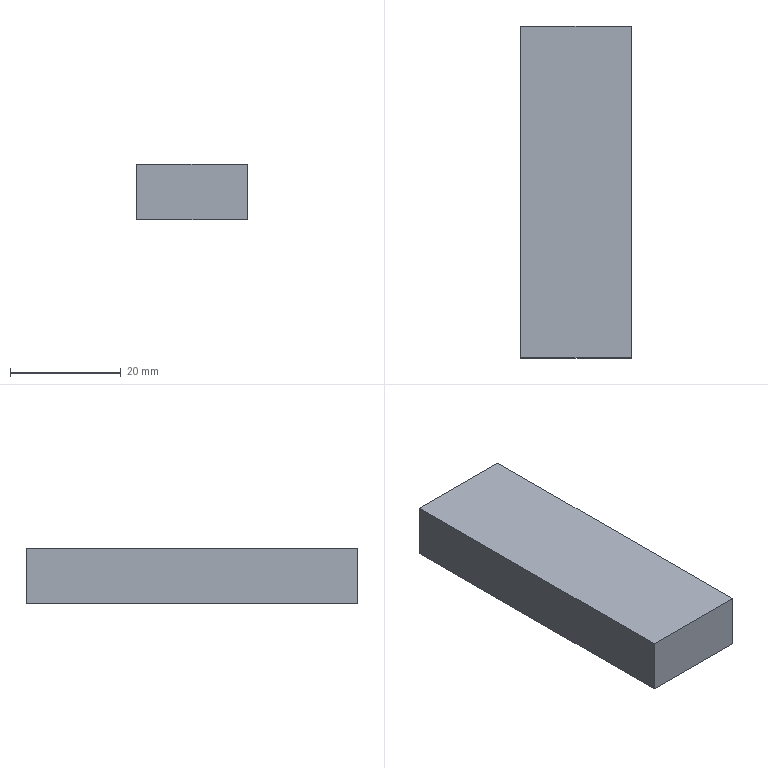Part | SolidWorks | features ICE 2, Extrusion 1 | 1 solid | 6 faces | box 20 x 60 x 10 mm | volume 12000 mm3 | plane 6
STEP:
#1=CARTESIAN_POINT('',(0.,0.,0.));
#2=VERTEX_POINT('',#1);
#3=CARTESIAN_POINT('',(20.,0.,0.));
#4=VERTEX_POINT('',#3);
#5=CARTESIAN_POINT('',(150.,0.,0.));
#6=DIRECTION('',(1.,0.,0.));
#7=VECTOR('',#6,1000.);
#8=LINE('',#5,#7);
#9=EDGE_CURVE('',#2,#4,#8,.T.);
#10=ORIENTED_EDGE('',*,*,#9,.T.);
#11=CARTESIAN_POINT('',(20.,0.,10.));
#12=VERTEX_POINT('',#11);
#13=CARTESIAN_POINT('',(20.,0.,0.));
#14=DIRECTION('',(0.,0.,1.));
#15=VECTOR('',#14,1000.);
#16=LINE('',#13,#15);
#17=EDGE_CURVE('',#4,#12,#16,.T.);
#18=ORIENTED_EDGE('',*,*,#17,.T.);
#19=CARTESIAN_POINT('',(0.,0.,10.));
#20=VERTEX_POINT('',#19);
#21=CARTESIAN_POINT('',(150.,0.,10.));
#22=DIRECTION('',(1.,0.,0.));
#23=VECTOR('',#22,1000.);
#24=LINE('',#21,#23);
#25=EDGE_CURVE('',#20,#12,#24,.T.);
#26=ORIENTED_EDGE('',*,*,#25,.F.);
#27=CARTESIAN_POINT('',(0.,0.,10.));
#28=DIRECTION('',(0.,0.,-1.));
#29=VECTOR('',#28,1000.);
#30=LINE('',#27,#29);
#31=EDGE_CURVE('',#20,#2,#30,.T.);
#32=ORIENTED_EDGE('',*,*,#31,.T.);
#33=EDGE_LOOP('',(#10,#18,#26,#32));
#34=FACE_OUTER_BOUND('',#33,.T.);
#35=CARTESIAN_POINT('',(150.,0.,10.));
#36=DIRECTION('',(0.,1.,0.));
#37=DIRECTION('',(0.,0.,1.));
#38=AXIS2_PLACEMENT_3D('',#35,#36,#37);
#39=PLANE('',#38);
#40=ADVANCED_FACE('',(#34),#39,.F.);
#41=CARTESIAN_POINT('',(20.,60.,10.));
#42=VERTEX_POINT('',#41);
#43=CARTESIAN_POINT('',(0.,60.,10.));
#44=VERTEX_POINT('',#43);
#45=CARTESIAN_POINT('',(0.,60.,10.));
#46=DIRECTION('',(-1.,0.,0.));
#47=VECTOR('',#46,1000.);
#48=LINE('',#45,#47);
#49=EDGE_CURVE('',#42,#44,#48,.T.);
#50=ORIENTED_EDGE('',*,*,#49,.F.);
#51=CARTESIAN_POINT('',(20.,60.,0.));
#52=VERTEX_POINT('',#51);
#53=CARTESIAN_POINT('',(20.,60.,0.));
#54=DIRECTION('',(0.,0.,1.));
#55=VECTOR('',#54,1000.);
#56=LINE('',#53,#55);
#57=EDGE_CURVE('',#52,#42,#56,.T.);
#58=ORIENTED_EDGE('',*,*,#57,.F.);
#59=CARTESIAN_POINT('',(0.,60.,0.));
#60=VERTEX_POINT('',#59);
#61=CARTESIAN_POINT('',(0.,60.,0.));
#62=DIRECTION('',(-1.,0.,0.));
#63=VECTOR('',#62,1000.);
#64=LINE('',#61,#63);
#65=EDGE_CURVE('',#52,#60,#64,.T.);
#66=ORIENTED_EDGE('',*,*,#65,.T.);
#67=CARTESIAN_POINT('',(0.,60.,10.));
#68=DIRECTION('',(0.,0.,-1.));
#69=VECTOR('',#68,1000.);
#70=LINE('',#67,#69);
#71=EDGE_CURVE('',#44,#60,#70,.T.);
#72=ORIENTED_EDGE('',*,*,#71,.F.);
#73=EDGE_LOOP('',(#50,#58,#66,#72));
#74=FACE_OUTER_BOUND('',#73,.T.);
#75=CARTESIAN_POINT('',(0.,60.,10.));
#76=DIRECTION('',(0.,-1.,0.));
#77=DIRECTION('',(0.,0.,-1.));
#78=AXIS2_PLACEMENT_3D('',#75,#76,#77);
#79=PLANE('',#78);
#80=ADVANCED_FACE('',(#74),#79,.F.);
#81=ORIENTED_EDGE('',*,*,#25,.T.);
#82=CARTESIAN_POINT('',(20.,0.,10.));
#83=DIRECTION('',(0.,-1.,0.));
#84=VECTOR('',#83,1000.);
#85=LINE('',#82,#84);
#86=EDGE_CURVE('',#42,#12,#85,.T.);
#87=ORIENTED_EDGE('',*,*,#86,.F.);
#88=ORIENTED_EDGE('',*,*,#49,.T.);
#89=CARTESIAN_POINT('',(0.,0.,10.));
#90=DIRECTION('',(0.,-1.,0.));
#91=VECTOR('',#90,1000.);
#92=LINE('',#89,#91);
#93=EDGE_CURVE('',#44,#20,#92,.T.);
#94=ORIENTED_EDGE('',*,*,#93,.T.);
#95=EDGE_LOOP('',(#81,#87,#88,#94));
#96=FACE_OUTER_BOUND('',#95,.T.);
#97=CARTESIAN_POINT('',(0.,0.,10.));
#98=DIRECTION('',(0.,0.,-1.));
#99=DIRECTION('',(-1.,0.,0.));
#100=AXIS2_PLACEMENT_3D('',#97,#98,#99);
#101=PLANE('',#100);
#102=ADVANCED_FACE('',(#96),#101,.F.);
#103=CARTESIAN_POINT('',(20.,0.,0.));
#104=DIRECTION('',(0.,-1.,0.));
#105=VECTOR('',#104,1000.);
#106=LINE('',#103,#105);
#107=EDGE_CURVE('',#52,#4,#106,.T.);
#108=ORIENTED_EDGE('',*,*,#107,.T.);
#109=ORIENTED_EDGE('',*,*,#9,.F.);
#110=CARTESIAN_POINT('',(0.,0.,0.));
#111=DIRECTION('',(0.,-1.,0.));
#112=VECTOR('',#111,1000.);
#113=LINE('',#110,#112);
#114=EDGE_CURVE('',#60,#2,#113,.T.);
#115=ORIENTED_EDGE('',*,*,#114,.F.);
#116=ORIENTED_EDGE('',*,*,#65,.F.);
#117=EDGE_LOOP('',(#108,#109,#115,#116));
#118=FACE_OUTER_BOUND('',#117,.T.);
#119=CARTESIAN_POINT('',(0.,0.,0.));
#120=DIRECTION('',(0.,0.,-1.));
#121=DIRECTION('',(-1.,0.,0.));
#122=AXIS2_PLACEMENT_3D('',#119,#120,#121);
#123=PLANE('',#122);
#124=ADVANCED_FACE('',(#118),#123,.T.);
#125=ORIENTED_EDGE('',*,*,#114,.T.);
#126=ORIENTED_EDGE('',*,*,#31,.F.);
#127=ORIENTED_EDGE('',*,*,#93,.F.);
#128=ORIENTED_EDGE('',*,*,#71,.T.);
#129=EDGE_LOOP('',(#125,#126,#127,#128));
#130=FACE_OUTER_BOUND('',#129,.T.);
#131=CARTESIAN_POINT('',(0.,0.,10.));
#132=DIRECTION('',(1.,0.,0.));
#133=DIRECTION('',(0.,0.,-1.));
#134=AXIS2_PLACEMENT_3D('',#131,#132,#133);
#135=PLANE('',#134);
#136=ADVANCED_FACE('',(#130),#135,.F.);
#137=ORIENTED_EDGE('',*,*,#86,.T.);
#138=ORIENTED_EDGE('',*,*,#17,.F.);
#139=ORIENTED_EDGE('',*,*,#107,.F.);
#140=ORIENTED_EDGE('',*,*,#57,.T.);
#141=EDGE_LOOP('',(#137,#138,#139,#140));
#142=FACE_OUTER_BOUND('',#141,.T.);
#143=CARTESIAN_POINT('',(20.,0.,0.));
#144=DIRECTION('',(-1.,0.,0.));
#145=DIRECTION('',(0.,0.,1.));
#146=AXIS2_PLACEMENT_3D('',#143,#144,#145);
#147=PLANE('',#146);
#148=ADVANCED_FACE('',(#142),#147,.F.);
#149=CLOSED_SHELL('',(#40,#80,#102,#124,#136,#148));
#150=MANIFOLD_SOLID_BREP('',#149);
#151=CARTESIAN_POINT('',(0.,0.,0.));
#152=DIRECTION('',(0.,0.,1.));
#153=DIRECTION('',(1.,0.,0.));
#154=AXIS2_PLACEMENT_3D('',#151,#152,#153);
#155=(LENGTH_UNIT()NAMED_UNIT(*)SI_UNIT(.MILLI.,.METRE.));
#156=UNCERTAINTY_MEASURE_WITH_UNIT(LENGTH_MEASURE(0.00001),#155,'','');
#157=(NAMED_UNIT(*)PLANE_ANGLE_UNIT()SI_UNIT($,.RADIAN.));
#158=(NAMED_UNIT(*)SI_UNIT($,.STERADIAN.)SOLID_ANGLE_UNIT());
#159=(GEOMETRIC_REPRESENTATION_CONTEXT(3)GLOBAL_UNCERTAINTY_ASSIGNED_CONTEXT((#156))GLOBAL_UNIT_ASSIGNED_CONTEXT((#155,#157,#158))REPRESENTATION_CONTEXT('',''));
#160=ADVANCED_BREP_SHAPE_REPRESENTATION('',(#150,#154),#159);